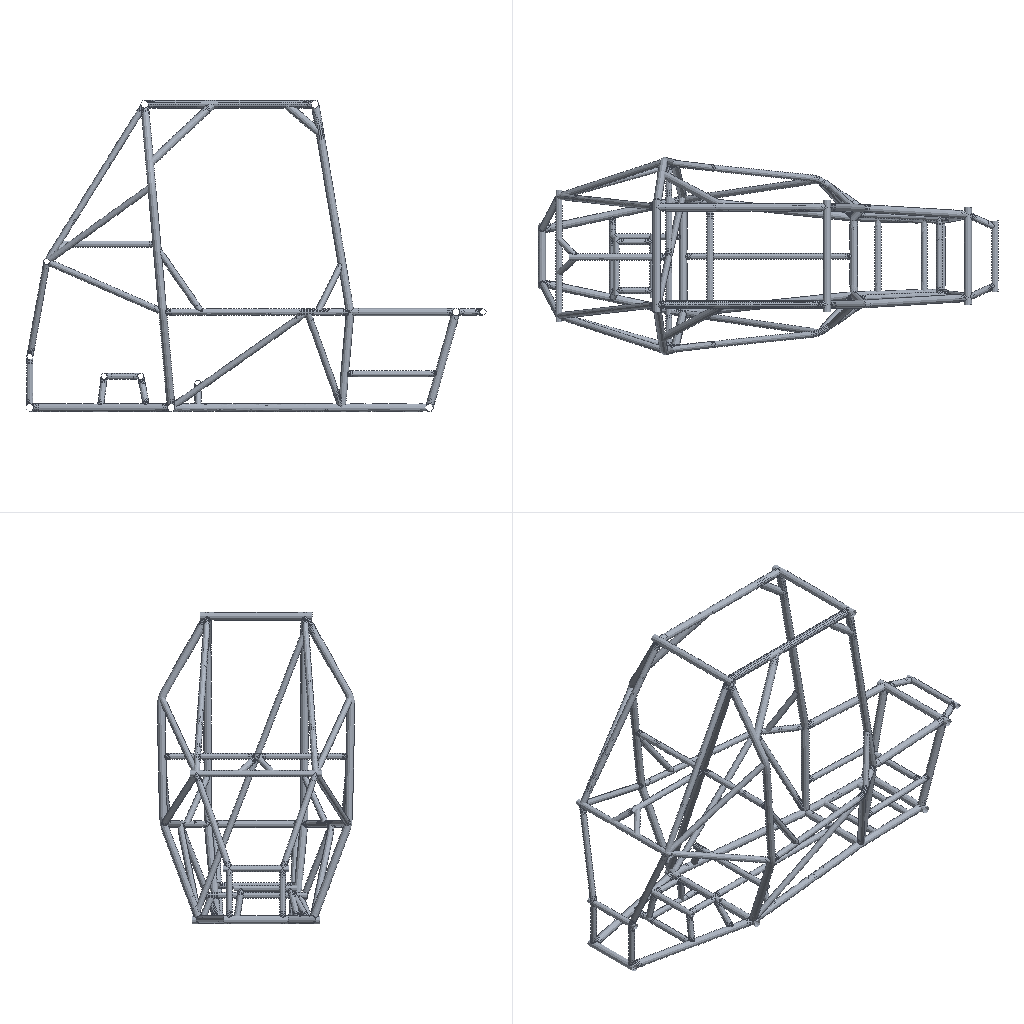Simulation study | ansys workbench
Set-up summary, first 98 of 221 lines:
category,name,step,type,value,unit,region
solver,ansys_workbench
units,mm-N-s-tonne (MPa),,stated,"/units,MPA"
analysis,LS1,,static
load_step,LS1,LS1,static,nsubst=1; time=1
mesh,nodes,,,59682
mesh,elements,,,95620
element_type,SHELL181,,,58416
element_type,CONTA174,,,18770
element_type,TARGE170,,,18398
element_type,CONTA177,,,36
material,4130?,,E,20500,tonne s^-2 mm^-1
material,4130?,,nu,0.29
material,4130?,,density,7.85e-09,tonne mm^-3
bc,"Elements for Body 1 ""fenxichejia0703-FreeParts|NONE""",model,fixed,[dofs=ALL n=3],,node list
bc,"Elements for Body 2 ""fenxichejia0703-FreeParts|NONE[2]""",model,fixed,[dofs=ALL n=3],,node list
bc,"Elements for Body 3 ""fenxichejia0703-FreeParts|NONE[3]""",model,fixed,[dofs=ALL n=3],,node list
bc,"Elements for Body 4 ""fenxichejia0703-FreeParts|NONE[4]""",model,fixed,[dofs=ALL n=3],,node list
bc,"Elements for Body 5 ""fenxichejia0703-FreeParts|NONE[5]""",model,fixed,[dofs=ALL n=3],,node list
bc,"Elements for Body 6 ""fenxichejia0703-FreeParts|NONE[6]""",model,fixed,[dofs=ALL n=3],,node list
bc,"Elements for Body 7 ""fenxichejia0703-FreeParts|NONE[7]""",model,fixed,[dofs=ALL n=3],,node list
bc,"Elements for Body 8 ""fenxichejia0703-FreeParts|NONE[8]""",model,fixed,[dofs=ALL n=3],,node list
bc,"Elements for Body 9 ""fenxichejia0703-FreeParts|NONE[9]""",model,fixed,[dofs=ALL n=3],,node list
bc,"Elements for Body 10 ""fenxichejia0703-FreeParts|NONE[10]""",model,fixed,[dofs=ALL n=3],,node list
bc,"Elements for Body 11 ""fenxichejia0703-FreeParts|NONE[11]""",model,fixed,[dofs=ALL n=3],,node list
bc,"Elements for Body 12 ""fenxichejia0703-FreeParts|NONE[12]""",model,fixed,[dofs=ALL n=3],,node list
bc,"Elements for Body 13 ""fenxichejia0703-FreeParts|NONE[13]""",model,fixed,[dofs=ALL n=3],,node list
bc,"Elements for Body 14 ""fenxichejia0703-FreeParts|NONE[14]""",model,fixed,[dofs=ALL n=3],,node list
bc,"Elements for Body 15 ""fenxichejia0703-FreeParts|NONE[15]""",model,fixed,[dofs=ALL n=3],,node list
bc,"Elements for Body 16 ""fenxichejia0703-FreeParts|NONE[16]""",model,fixed,[dofs=ALL n=3],,node list
bc,"Elements for Body 17 ""fenxichejia0703-FreeParts|NONE[17]""",model,fixed,[dofs=ALL n=3],,node list
bc,"Elements for Body 18 ""fenxichejia0703-FreeParts|NONE[18]""",model,fixed,[dofs=ALL n=3],,node list
bc,"Elements for Body 19 ""fenxichejia0703-FreeParts|NONE[19]""",model,fixed,[dofs=ALL n=3],,node list
bc,"Elements for Body 20 ""fenxichejia0703-FreeParts|NONE[20]""",model,fixed,[dofs=ALL n=3],,node list
bc,"Elements for Body 21 ""fenxichejia0703-FreeParts|NONE[21]""",model,fixed,[dofs=ALL n=3],,node list
bc,"Elements for Body 22 ""fenxichejia0703-FreeParts|NONE[22]""",model,fixed,[dofs=ALL n=3],,node list
bc,"Elements for Body 23 ""fenxichejia0703-FreeParts|NONE[23]""",model,fixed,[dofs=ALL n=3],,node list
bc,"Elements for Body 24 ""fenxichejia0703-FreeParts|NONE[24]""",model,fixed,[dofs=ALL n=3],,node list
bc,"Elements for Body 25 ""fenxichejia0703-FreeParts|NONE[25]""",model,fixed,[dofs=ALL n=3],,node list
bc,"Elements for Body 26 ""fenxichejia0703-FreeParts|NONE[26]""",model,fixed,[dofs=ALL n=3],,node list
bc,"Elements for Body 27 ""fenxichejia0703-FreeParts|NONE[27]""",model,fixed,[dofs=ALL n=3],,node list
bc,"Elements for Body 28 ""fenxichejia0703-FreeParts|NONE[28]""",model,fixed,[dofs=ALL n=3],,node list
bc,"Elements for Body 29 ""fenxichejia0703-FreeParts|NONE[29]""",model,fixed,[dofs=ALL n=3],,node list
bc,"Elements for Body 30 ""fenxichejia0703-FreeParts|NONE[30]""",model,fixed,[dofs=ALL n=3],,node list
bc,"Elements for Body 31 ""fenxichejia0703-FreeParts|NONE[31]""",model,fixed,[dofs=ALL n=3],,node list
bc,"Elements for Body 32 ""fenxichejia0703-FreeParts|NONE[32]""",model,fixed,[dofs=ALL n=3],,node list
bc,"Elements for Body 33 ""fenxichejia0703-FreeParts|NONE[33]""",model,fixed,[dofs=ALL n=3],,node list
bc,"Elements for Body 34 ""fenxichejia0703-FreeParts|NONE[34]""",model,fixed,[dofs=ALL n=3],,node list
bc,"Elements for Body 35 ""fenxichejia0703-FreeParts|NONE[35]""",model,fixed,[dofs=ALL n=3],,node list
bc,"Elements for Body 36 ""fenxichejia0703-FreeParts|NONE[36]""",model,fixed,[dofs=ALL n=3],,node list
bc,"Elements for Body 37 ""fenxichejia0703-FreeParts|NONE[37]""",model,fixed,[dofs=ALL n=3],,node list
bc,"Elements for Body 38 ""fenxichejia0703-FreeParts|NONE[38]""",model,fixed,[dofs=ALL n=3],,node list
bc,"Elements for Body 39 ""fenxichejia0703-FreeParts|NONE[39]""",model,fixed,[dofs=ALL n=3],,node list
bc,"Elements for Body 40 ""fenxichejia0703-FreeParts|NONE[40]""",model,fixed,[dofs=ALL n=3],,node list
bc,"Elements for Body 41 ""fenxichejia0703-FreeParts|NONE[41]""",model,fixed,[dofs=ALL n=3],,node list
bc,"Elements for Body 42 ""fenxichejia0703-FreeParts|NONE[42]""",model,fixed,[dofs=ALL n=3],,node list
bc,"Elements for Body 43 ""fenxichejia0703-FreeParts|NONE[43]""",model,fixed,[dofs=ALL n=3],,node list
bc,"Elements for Body 44 ""fenxichejia0703-FreeParts|NONE[44]""",model,fixed,[dofs=ALL n=3],,node list
bc,"Elements for Body 45 ""fenxichejia0703-FreeParts|NONE[45]""",model,fixed,[dofs=ALL n=3],,node list
bc,"Elements for Body 46 ""fenxichejia0703-FreeParts|NONE[46]""",model,fixed,[dofs=ALL n=3],,node list
bc,"Elements for Body 47 ""fenxichejia0703-FreeParts|NONE[47]""",model,fixed,[dofs=ALL n=3],,node list
bc,"Elements for Body 48 ""fenxichejia0703-FreeParts|NONE[48]""",model,fixed,[dofs=ALL n=3],,node list
bc,"Elements for Body 49 ""fenxichejia0703-FreeParts|NONE[49]""",model,fixed,[dofs=ALL n=3],,node list
bc,"Elements for Body 50 ""fenxichejia0703-FreeParts|NONE[50]""",model,fixed,[dofs=ALL n=3],,node list
bc,"Elements for Body 51 ""fenxichejia0703-FreeParts|NONE[51]""",model,fixed,[dofs=ALL n=3],,node list
bc,"Elements for Body 52 ""fenxichejia0703-FreeParts|NONE[52]""",model,fixed,[dofs=ALL n=3],,node list
bc,"Elements for Body 53 ""fenxichejia0703-FreeParts|NONE[53]""",model,fixed,[dofs=ALL n=3],,node list
bc,"Elements for Body 54 ""fenxichejia0703-FreeParts|NONE[54]""",model,fixed,[dofs=ALL n=3],,node list
bc,"Elements for Body 55 ""fenxichejia0703-FreeParts|NONE[55]""",model,fixed,[dofs=ALL n=3],,node list
bc,"Elements for Body 56 ""fenxichejia0703-FreeParts|NONE[56]""",model,fixed,[dofs=ALL n=3],,node list
bc,"Elements for Body 57 ""fenxichejia0703-FreeParts|NONE[57]""",model,fixed,[dofs=ALL n=3],,node list
bc,"Elements for Body 58 ""fenxichejia0703-FreeParts|NONE[58]""",model,fixed,[dofs=ALL n=3],,node list
bc,"Elements for Body 59 ""fenxichejia0703-FreeParts|NONE[59]""",model,fixed,[dofs=ALL n=3],,node list
bc,"Elements for Body 60 ""fenxichejia0703-FreeParts|NONE[60]""",model,fixed,[dofs=ALL n=3],,node list
bc,"Elements for Body 61 ""fenxichejia0703-FreeParts|NONE[61]""",model,fixed,[dofs=ALL n=3],,node list
bc,"Elements for Body 62 ""fenxichejia0703-FreeParts|NONE[62]""",model,fixed,[dofs=ALL n=3],,node list
bc,"Elements for Body 63 ""fenxichejia0703-FreeParts|NONE[63]""",model,fixed,[dofs=ALL n=3],,node list
bc,"Elements for Body 64 ""fenxichejia0703-FreeParts|NONE[64]""",model,fixed,[dofs=ALL n=3],,node list
bc,"Elements for Body 65 ""fenxichejia0703-FreeParts|NONE[65]""",model,fixed,[dofs=ALL n=3],,node list
bc,"Elements for Body 66 ""fenxichejia0703-FreeParts|NONE[66]""",model,fixed,[dofs=ALL n=3],,node list
bc,"Elements for Body 67 ""fenxichejia0703-FreeParts|NONE[67]""",model,fixed,[dofs=ALL n=3],,node list
bc,"Elements for Body 68 ""fenxichejia0703-FreeParts|NONE[68]""",model,fixed,[dofs=ALL n=3],,node list
bc,"Elements for Body 69 ""fenxichejia0703-FreeParts|NONE[69]""",model,fixed,[dofs=ALL n=3],,node list
bc,"Elements for Body 70 ""fenxichejia0703-FreeParts|NONE[70]""",model,fixed,[dofs=ALL n=3],,node list
bc,"Elements for Body 71 ""fenxichejia0703-FreeParts|NONE[71]""",model,fixed,[dofs=ALL n=3],,node list
bc,,LS1,prescribed uz,5 [dofs=UZ n=4],,node list
contact,Contact Region,,bonded (always),element=CONTA174
contact,Contact Region 2,,bonded (always),element=CONTA174
contact,Contact Region 3,,bonded (always),element=CONTA174
contact,Contact Region 4,,bonded (always),element=CONTA174
contact,Contact Region 5,,bonded (always),element=CONTA174
contact,Contact Region 6,,bonded (always),element=CONTA174
contact,Contact Region 7,,bonded (always),element=CONTA174
contact,Contact Region 8,,bonded (always),element=CONTA174
contact,Contact Region 9,,bonded (always),element=CONTA174
contact,Contact Region 10,,bonded (always),element=CONTA174
contact,Contact Region 11,,bonded (always),element=CONTA174
contact,Contact Region 12,,bonded (always),element=CONTA174
Ansys APDL input file, long lists of numbers shortened:
/batch
/config,noeldb,1     ! force off writing results to database
*get,_wallstrt,active,,time,wall
! ANSYS input file written by Workbench version 2021 R1
! File used for geometry attach:
/title,_______--____ (A5)
! ****** Begin Custom Load Command Snippet ******
/COM, ACT Extensions:
/COM,     LSDYNA, 2021.1
/COM,
! ****** End   Custom Load Command Snippet ******
*DIM,_wb_ProjectScratch_dir,string,248
_wb_ProjectScratch_dir(1) = ''
*DIM,_wb_SolverFiles_dir,string,248
_wb_SolverFiles_dir(1) = ''
*DIM,_wb_userfiles_dir,string,248
_wb_userfiles_dir(1) = ''
/com,--- Data in consistent NMM units. See Solving Units in the help system for more information.
/units,MPA
/nopr
/wb,file,start              !  signify a WB generated input file
/prep7
! Turn off shape checking because checks already performed inside WB mesher.
! See help system for more information.
SHPP,OFF,,NOWARN
/nolist
etcon,set             ! allow ANSYS to choose best KEYOP's for 180x elements, resets any applicable keyopt to MAPDL defaults
/com,*********** Nodes for the whole assembly ***********
nblock,3,,65645
(1i9,3e20.9e3)
        1     1.226998401E+02     1.799362606E+02     1.000000019E+02
! (59677 more lines like these left out)
-1
/com,*********** Nodes for all Remote Points ***********
nblock,3
(1i9,3e20.9e3)
    59679    -5.800208747E+02    -1.300000000E+02     6.838973832E-14
    59680    -5.800208747E+02     1.300000000E+02    -4.884981308E-14
    59681     1.060020881E+03    -1.800000000E+02    -2.451372438E-13
    59682     1.060020881E+03     1.800000000E+02     2.522426712E-13
-1
/wb,elem,start            !  set before creation of elements
/com,*********** Elements for Body 1 "fenxichejia0703-FreeParts|NONE" ***********
et,1,181
keyo,1,3,2
eblock,19,solid,,344
(19i9)
        1        1        1        1        0        0        0        0        4        0      199      457      341      467      467
! (343 more lines like these left out)
-1
/com,*********** Elements for Body 2 "fenxichejia0703-FreeParts|NONE[2]" ***********
et,2,181
keyo,2,3,2
eblock,19,solid,,220
(19i9)
        2        2        2        2        0        0        0        0        4        0     2766     2885     2887     3082     3082
! (219 more lines like these left out)
-1
/com,*********** Elements for Body 3 "fenxichejia0703-FreeParts|NONE[3]" ***********
et,3,181
keyo,3,3,2
eblock,19,solid,,992
(19i9)
        3        3        3        3        0        0        0        0        4        0    39705    41781    41416    41519    41419
! (991 more lines like these left out)
-1
/com,*********** Elements for Body 4 "fenxichejia0703-FreeParts|NONE[4]" ***********
et,4,181
keyo,4,3,2
eblock,19,solid,,978
(19i9)
        4        4        4        4        0        0        0        0        4        0    41902    43622    43598    43712    43712
! (977 more lines like these left out)
-1
/com,*********** Elements for Body 5 "fenxichejia0703-FreeParts|NONE[5]" ***********
et,5,181
keyo,5,3,2
eblock,19,solid,,572
(19i9)
        5        5        5        5        0        0        0        0        4        0    19833    20845    20860    20630    20630
! (571 more lines like these left out)
-1
! (66 more sections like these left out)
/wb,elem,end               !  done creating elements
/com,*********** Send User Defined Coordinate System(s) ***********
csys,0
toffst,273.15,  ! Temperature offset from absolute zero
/com,*********** Set Reference Temperature ***********
tref,22.
/wb,mat,start              !  starting to send materials
/com,*********** Send Materials ***********
MP,DENS,1,7.85e-09,	! tonne mm^-3
MP,EX,1,20500,	! tonne s^-2 mm^-1
MP,NUXY,1,0.29,
MP,DENS,2,7.85e-09,	! tonne mm^-3
! (209 more lines like these left out)
/wb,mat,end                !  done sending materials
/com,*********** Send Sheet Properties ***********
sectype,29,shell
secdata,3.
secoff,mid
sectype,30,shell
secdata,3.
secoff,mid
sectype,31,shell
secdata,3.
secoff,mid
sectype,32,shell
secdata,3.
secoff,mid
sectype,33,shell
secdata,3.
secoff,mid
sectype,34,shell
secdata,3.
secoff,mid
sectype,35,shell
secdata,3.
secoff,mid
sectype,36,shell
secdata,3.
secoff,mid
sectype,37,shell
secdata,3.
secoff,mid
sectype,38,shell
secdata,3.
secoff,mid
sectype,39,shell
secdata,3.
secoff,mid
sectype,40,shell
secdata,3.
secoff,mid
sectype,41,shell
secdata,3.
secoff,mid
sectype,42,shell
secdata,3.
secoff,mid
sectype,43,shell
secdata,3.
secoff,mid
sectype,44,shell
secdata,3.
secoff,mid
sectype,45,shell
secdata,3.
secoff,mid
sectype,46,shell
secdata,3.
secoff,mid
sectype,47,shell
secdata,3.
secoff,mid
sectype,48,shell
secdata,3.
secoff,mid
sectype,49,shell
secdata,3.
secoff,mid
sectype,50,shell
secdata,3.
secoff,mid
sectype,51,shell
secdata,3.
secoff,mid
sectype,1,shell
secdata,3.
secoff,mid
sectype,52,shell
secdata,3.
secoff,mid
sectype,53,shell
secdata,3.
secoff,mid
sectype,54,shell
! (147 more lines like these left out)
/wb,contact,start          !  starting to send contact
/com,*********** Create Contact "接触区域" ***********
/com,            Real Constant Set For Above Contact Is 73 & 72
*set,tid,73
*set,cid,72
r,tid
r,cid
et,tid,170
et,cid,174
eblock,10,,,78
(15i9)
    58421       73       73       73        0      277      283      285      285
! (77 more lines like these left out)
-1
eblock,10,,,78
(15i9)
    58499       72       72       72        0      277      283      285      285
! (77 more lines like these left out)
-1
eblock,10,,,40
(15i9)
    58577       72       73       72        0     3112     3043     3046     3046
! (39 more lines like these left out)
-1
eblock,10,,,40
(15i9)
    58617       73       72       73        0     3112     3043     3046     3046
! (39 more lines like these left out)
-1
keyo,cid,8,2               ! auto create asymmetric contact (from Program Controlled setting)
keyo,cid,10,0              ! adjust contact stiffness each NR iteration (from Program Controlled setting)
keyo,cid,12,5              ! bonded always
keyo,cid,18,1              ! small sliding turned on by application
keyo,cid,2,0               ! augmented Lagrange (from Program Controlled setting)
keyo,cid,4,0               ! on Gauss point (from Program Controlled setting)
keyo,cid,9,1               ! ignore initial gaps/penetration
keyo,cid,7,0               ! No Prediction
rmod,tid,3,10.      ! FKN
rmod,tid,5,0.       ! ICONT
rmod,tid,6,-6.067  ! PINB
rmod,tid,10,0.      ! CNOF
rmod,tid,12,0.      ! FKT
rmod,tid,36,234     ! WB DSID
rmod,cid,3,10.      ! FKN
rmod,cid,5,0.       ! ICONT
rmod,cid,6,-6.067  ! PINB
rmod,cid,10,0.      ! CNOF
rmod,cid,12,0.      ! FKT
rmod,cid,36,234     ! WB DSID
/com,*********** Create Contact "接触区域 2" ***********
/com,            Real Constant Set For Above Contact Is 75 & 74
*set,tid,75
*set,cid,74
r,tid
r,cid
et,tid,170
et,cid,174
eblock,10,,,41
(15i9)
    58657       75       75       75        0      464      383      326      327
! (40 more lines like these left out)
-1
eblock,10,,,41
(15i9)
    58698       74       74       74        0      464      383      326      327
! (40 more lines like these left out)
-1
eblock,10,,,32
(15i9)
    58739       74       75       74        0    23870    24089    23860    24099
! (31 more lines like these left out)
-1
eblock,10,,,32
(15i9)
    58771       75       74       75        0    23870    24089    23860    24099
! (31 more lines like these left out)
-1
keyo,cid,8,2               ! auto create asymmetric contact (from Program Controlled setting)
keyo,cid,10,0              ! adjust contact stiffness each NR iteration (from Program Controlled setting)
keyo,cid,12,5              ! bonded always
keyo,cid,18,1              ! small sliding turned on by application
keyo,cid,2,0               ! augmented Lagrange (from Program Controlled setting)
keyo,cid,4,0               ! on Gauss point (from Program Controlled setting)
keyo,cid,9,1               ! ignore initial gaps/penetration
keyo,cid,7,0               ! No Prediction
rmod,tid,3,10.      ! FKN
rmod,tid,5,0.       ! ICONT
rmod,tid,6,-6.067  ! PINB
rmod,tid,10,0.      ! CNOF
rmod,tid,12,0.      ! FKT
rmod,tid,36,237     ! WB DSID
rmod,cid,3,10.      ! FKN
rmod,cid,5,0.       ! ICONT
rmod,cid,6,-6.067  ! PINB
rmod,cid,10,0.      ! CNOF
rmod,cid,12,0.      ! FKT
rmod,cid,36,237     ! WB DSID
/com,*********** Create Contact "接触区域 3" ***********
/com,            Real Constant Set For Above Contact Is 77 & 76
*set,tid,77
*set,cid,76
r,tid
r,cid
et,tid,170
et,cid,174
eblock,10,,,76
(15i9)
    58803       77       77       77        0      226      225      228      228
! (75 more lines like these left out)
-1
eblock,10,,,76
(15i9)
    58879       76       76       76        0      226      225      228      228
! (75 more lines like these left out)
-1
eblock,10,,,111
(15i9)
    58955       76       77       76        0    35492    35870    35666    35665
! (110 more lines like these left out)
-1
eblock,10,,,111
(15i9)
    59066       77       76       77        0    35492    35870    35666    35665
! (110 more lines like these left out)
-1
keyo,cid,8,2               ! auto create asymmetric contact (from Program Controlled setting)
keyo,cid,10,0              ! adjust contact stiffness each NR iteration (from Program Controlled setting)
keyo,cid,12,5              ! bonded always
keyo,cid,18,1              ! small sliding turned on by application
keyo,cid,2,0               ! augmented Lagrange (from Program Controlled setting)
keyo,cid,4,0               ! on Gauss point (from Program Controlled setting)
keyo,cid,9,1               ! ignore initial gaps/penetration
keyo,cid,7,0               ! No Prediction
rmod,tid,3,10.      ! FKN
rmod,tid,5,0.       ! ICONT
rmod,tid,6,-6.067  ! PINB
rmod,tid,10,0.      ! CNOF
rmod,tid,12,0.      ! FKT
rmod,tid,36,240     ! WB DSID
rmod,cid,3,10.      ! FKN
rmod,cid,5,0.       ! ICONT
rmod,cid,6,-6.067  ! PINB
rmod,cid,10,0.      ! CNOF
rmod,cid,12,0.      ! FKT
rmod,cid,36,240     ! WB DSID
/com,*********** Create Contact "接触区域 4" ***********
/com,            Real Constant Set For Above Contact Is 79 & 78
*set,tid,79
*set,cid,78
r,tid
r,cid
et,tid,170
et,cid,174
eblock,10,,,70
(15i9)
    59177       79       79       79        0     3112     3043     3046     3046
! (69 more lines like these left out)
-1
eblock,10,,,70
(15i9)
    59247       78       78       78        0     3112     3043     3046     3046
! (69 more lines like these left out)
-1
eblock,10,,,88
(15i9)
    59317       78       79       78        0    24115    24398    24187    24186
! (87 more lines like these left out)
-1
eblock,10,,,88
(15i9)
    59405       79       78       79        0    24115    24398    24187    24186
! (87 more lines like these left out)
-1
keyo,cid,8,2               ! auto create asymmetric contact (from Program Controlled setting)
keyo,cid,10,0              ! adjust contact stiffness each NR iteration (from Program Controlled setting)
keyo,cid,12,5              ! bonded always
keyo,cid,18,1              ! small sliding turned on by application
keyo,cid,2,0               ! augmented Lagrange (from Program Controlled setting)
keyo,cid,4,0               ! on Gauss point (from Program Controlled setting)
keyo,cid,9,1               ! ignore initial gaps/penetration
keyo,cid,7,0               ! No Prediction
rmod,tid,3,10.      ! FKN
rmod,tid,5,0.       ! ICONT
rmod,tid,6,-6.067  ! PINB
rmod,tid,10,0.      ! CNOF
rmod,tid,12,0.      ! FKT
rmod,tid,36,243     ! WB DSID
rmod,cid,3,10.      ! FKN
rmod,cid,5,0.       ! ICONT
rmod,cid,6,-6.067  ! PINB
rmod,cid,10,0.      ! CNOF
rmod,cid,12,0.      ! FKT
rmod,cid,36,243     ! WB DSID
/com,*********** Create Contact "接触区域 5" ***********
/com,            Real Constant Set For Above Contact Is 81 & 80
*set,tid,81
*set,cid,80
r,tid
r,cid
et,tid,170
et,cid,174
eblock,10,,,68
(15i9)
    59493       81       81       81        0     2885     2887     3082     3082
! (67 more lines like these left out)
-1
eblock,10,,,68
(15i9)
    59561       80       80       80        0     2885     2887     3082     3082
! (67 more lines like these left out)
-1
eblock,10,,,106
(15i9)
    59629       80       81       80        0    35489    35493    35589    35588
! (105 more lines like these left out)
-1
eblock,10,,,106
(15i9)
    59735       81       80       81        0    35489    35493    35589    35588
! (105 more lines like these left out)
-1
keyo,cid,8,2               ! auto create asymmetric contact (from Program Controlled setting)
keyo,cid,10,0              ! adjust contact stiffness each NR iteration (from Program Controlled setting)
keyo,cid,12,5              ! bonded always
keyo,cid,18,1              ! small sliding turned on by application
keyo,cid,2,0               ! augmented Lagrange (from Program Controlled setting)
keyo,cid,4,0               ! on Gauss point (from Program Controlled setting)
keyo,cid,9,1               ! ignore initial gaps/penetration
keyo,cid,7,0               ! No Prediction
rmod,tid,3,10.      ! FKN
rmod,tid,5,0.       ! ICONT
rmod,tid,6,-6.067  ! PINB
rmod,tid,10,0.      ! CNOF
rmod,tid,12,0.      ! FKT
rmod,tid,36,246     ! WB DSID
rmod,cid,3,10.      ! FKN
rmod,cid,5,0.       ! ICONT
rmod,cid,6,-6.067  ! PINB
rmod,cid,10,0.      ! CNOF
rmod,cid,12,0.      ! FKT
rmod,cid,36,246     ! WB DSID
! (125 more sections like these left out)
/wb,contact,end            !  done creating contacts
/golist
/wb,load,start             !  starting to send loads
/com,*********** Create Remote Point "内部远程点" ***********
! -------- Remote Point Used by "远程位移" --------
*set,tid,333
*set,cid,332
et,cid,174
et,tid,170
keyo,tid,2,1               ! Don't fix the pilot node
keyo,tid,4,111111
keyo,cid,12,5              ! Bonded Contact
keyo,cid,4,1               ! Deformable RBE3 style load
keyo,cid,2,2               ! MPC style contact
eblock,10,,,372
(15i9)
    95217      332      332      332        0    15146    15183    15182    15145
! (371 more lines like these left out)
-1
*set,_npilot,59679
_npilot645=_npilot
type,tid
mat ,cid
real,cid
tshape,pilo
en,95589,_npilot
tshape
/com,*********** Create Remote Point "内部远程点 2" ***********
! -------- Remote Point Used by "远程位移 2" --------
*set,tid,335
*set,cid,334
et,cid,177
et,tid,170
keyo,tid,2,1               ! Don't fix the pilot node
keyo,tid,4,111111
keyo,cid,12,5              ! Bonded Contact
keyo,cid,4,1               ! Deformable RBE3 style load
keyo,cid,2,2               ! MPC style contact
eblock,10,,,12
(15i9)
    95590      334      334      334        0    15093    15135
! (11 more lines like these left out)
-1
*set,_npilot,59680
_npilot657=_npilot
type,tid
mat ,cid
real,cid
tshape,pilo
en,95602,_npilot
tshape
/com,*********** Create Remote Point "内部远程点 3" ***********
! -------- Remote Point Used by "远程位移 3" --------
*set,tid,337
*set,cid,336
et,cid,177
et,tid,170
keyo,tid,2,1               ! Don't fix the pilot node
keyo,tid,4,111111
keyo,cid,12,5              ! Bonded Contact
keyo,cid,4,1               ! Deformable RBE3 style load
keyo,cid,2,2               ! MPC style contact
eblock,10,,,12
(15i9)
    95603      336      336      336        0    16627    16680
! (11 more lines like these left out)
-1
*set,_npilot,59681
_npilot660=_npilot
type,tid
mat ,cid
real,cid
tshape,pilo
en,95615,_npilot
tshape
/com,*********** Create Remote Point "内部远程点 4" ***********
! -------- Remote Point Used by "远程位移 4" --------
*set,tid,339
*set,cid,338
et,cid,177
et,tid,170
keyo,tid,2,1               ! Don't fix the pilot node
keyo,tid,4,111111
keyo,cid,12,5              ! Bonded Contact
keyo,cid,4,1               ! Deformable RBE3 style load
keyo,cid,2,2               ! MPC style contact
eblock,10,,,12
(15i9)
    95616      338      338      338        0    16583    16685
! (11 more lines like these left out)
-1
*set,_npilot,59682
_npilot663=_npilot
type,tid
mat ,cid
real,cid
tshape,pilo
en,95628,_npilot
tshape
/com,*********** Construct Remote Displacement ***********
/com,*********** Construct Remote Displacement ***********
/com,*********** Construct Remote Displacement ***********
/com,*********** Construct Remote Displacement ***********
/COM,*** Create a component for all remote displacements ***
CMBLOCK,REMOTEDISPALL,NODE,        4
(8i10)
     59679     59680     59681     59682
et,340,14             ! spring element type
/com,*********** Construct Weak Springs, Prototype 1 ***********
*set,_delta,8.434
type,340
mat,341
real,341
r,341,9.98216507957579e-005
nsel,all
*get,_nspr,ndmx
_nspr=_nspr+1
esel,s,type,,1
nsle,s,active
*get,_minx,node,0,mnloc,x
*get,_miny,node,0,mnloc,y
*get,_minz,node,0,mnloc,z
*get,_maxx,node,0,mxloc,x
*get,_maxy,node,0,mxloc,y
*get,_maxz,node,0,mxloc,z
*dim,_ntets,arra,8
_ntets(1) = NODE(_minx,_miny,_minz)
_ntets(2) = NODE(_minx,_miny,_maxz)
_ntets(3) = NODE(_minx,_maxy,_minz)
_ntets(4) = NODE(_minx,_maxy,_maxz)
_ntets(5) = NODE(_maxx,_miny,_minz)
_ntets(6) = NODE(_maxx,_miny,_maxz)
_ntets(7) = NODE(_maxx,_maxy,_minz)
_ntets(8) = NODE(_maxx,_maxy,_maxz)
*do,_i,1,8
  n,_nspr,nx(_ntets(_i))+_delta,ny(_ntets(_i)),nz(_ntets(_i))
  e,_ntets(_i),_nspr
  d,_nspr,all
  _nspr=_nspr+1
  n,_nspr,nx(_ntets(_i)),ny(_ntets(_i))+_delta,nz(_ntets(_i))
  e,_ntets(_i),_nspr
  d,_nspr,all
  _nspr=_nspr+1
  n,_nspr,nx(_ntets(_i)),ny(_ntets(_i)),nz(_ntets(_i))+_delta
  e,_ntets(_i),_nspr
  d,_nspr,all
  _nspr=_nspr+1
*enddo
*set,_ntets
nsel,all
esel,all
/com,*********** Construct Weak Springs, Prototype 2 ***********
*set,_delta,8.259
type,340
mat,342
real,342
r,342,1.2338667019096e-004
nsel,all
*get,_nspr,ndmx
_nspr=_nspr+1
esel,s,type,,2
nsle,s,active
*get,_minx,node,0,mnloc,x
*get,_miny,node,0,mnloc,y
*get,_minz,node,0,mnloc,z
*get,_maxx,node,0,mxloc,x
*get,_maxy,node,0,mxloc,y
*get,_maxz,node,0,mxloc,z
*dim,_ntets,arra,8
_ntets(1) = NODE(_minx,_miny,_minz)
_ntets(2) = NODE(_minx,_miny,_maxz)
_ntets(3) = NODE(_minx,_maxy,_minz)
_ntets(4) = NODE(_minx,_maxy,_maxz)
_ntets(5) = NODE(_maxx,_miny,_minz)
_ntets(6) = NODE(_maxx,_miny,_maxz)
_ntets(7) = NODE(_maxx,_maxy,_minz)
_ntets(8) = NODE(_maxx,_maxy,_maxz)
*do,_i,1,8
  n,_nspr,nx(_ntets(_i))+_delta,ny(_ntets(_i)),nz(_ntets(_i))
  e,_ntets(_i),_nspr
  d,_nspr,all
  _nspr=_nspr+1
  n,_nspr,nx(_ntets(_i)),ny(_ntets(_i))+_delta,nz(_ntets(_i))
  e,_ntets(_i),_nspr
  d,_nspr,all
  _nspr=_nspr+1
  n,_nspr,nx(_ntets(_i)),ny(_ntets(_i)),nz(_ntets(_i))+_delta
  e,_ntets(_i),_nspr
  d,_nspr,all
  _nspr=_nspr+1
*enddo
*set,_ntets
nsel,all
esel,all
/com,*********** Construct Weak Springs, Prototype 3 ***********
*set,_delta,35.074
type,340
mat,343
real,343
r,343,1.68498675560958e-004
nsel,all
*get,_nspr,ndmx
_nspr=_nspr+1
esel,s,type,,3
nsle,s,active
*get,_minx,node,0,mnloc,x
*get,_miny,node,0,mnloc,y
*get,_minz,node,0,mnloc,z
*get,_maxx,node,0,mxloc,x
*get,_maxy,node,0,mxloc,y
*get,_maxz,node,0,mxloc,z
*dim,_ntets,arra,8
_ntets(1) = NODE(_minx,_miny,_minz)
_ntets(2) = NODE(_minx,_miny,_maxz)
_ntets(3) = NODE(_minx,_maxy,_minz)
_ntets(4) = NODE(_minx,_maxy,_maxz)
_ntets(5) = NODE(_maxx,_miny,_minz)
_ntets(6) = NODE(_maxx,_miny,_maxz)
_ntets(7) = NODE(_maxx,_maxy,_minz)
_ntets(8) = NODE(_maxx,_maxy,_maxz)
*do,_i,1,8
  n,_nspr,nx(_ntets(_i))+_delta,ny(_ntets(_i)),nz(_ntets(_i))
  e,_ntets(_i),_nspr
  d,_nspr,all
  _nspr=_nspr+1
  n,_nspr,nx(_ntets(_i)),ny(_ntets(_i))+_delta,nz(_ntets(_i))
  e,_ntets(_i),_nspr
  d,_nspr,all
  _nspr=_nspr+1
  n,_nspr,nx(_ntets(_i)),ny(_ntets(_i)),nz(_ntets(_i))+_delta
  e,_ntets(_i),_nspr
  d,_nspr,all
  _nspr=_nspr+1
*enddo
*set,_ntets
nsel,all
esel,all
/com,*********** Construct Weak Springs, Prototype 4 ***********
*set,_delta,35.074
type,340
mat,344
real,344
r,344,1.69411550265547e-004
nsel,all
*get,_nspr,ndmx
_nspr=_nspr+1
esel,s,type,,4
nsle,s,active
*get,_minx,node,0,mnloc,x
*get,_miny,node,0,mnloc,y
*get,_minz,node,0,mnloc,z
*get,_maxx,node,0,mxloc,x
*get,_maxy,node,0,mxloc,y
*get,_maxz,node,0,mxloc,z
*dim,_ntets,arra,8
_ntets(1) = NODE(_minx,_miny,_minz)
_ntets(2) = NODE(_minx,_miny,_maxz)
_ntets(3) = NODE(_minx,_maxy,_minz)
_ntets(4) = NODE(_minx,_maxy,_maxz)
_ntets(5) = NODE(_maxx,_miny,_minz)
_ntets(6) = NODE(_maxx,_miny,_maxz)
_ntets(7) = NODE(_maxx,_maxy,_minz)
_ntets(8) = NODE(_maxx,_maxy,_maxz)
*do,_i,1,8
  n,_nspr,nx(_ntets(_i))+_delta,ny(_ntets(_i)),nz(_ntets(_i))
  e,_ntets(_i),_nspr
  d,_nspr,all
  _nspr=_nspr+1
  n,_nspr,nx(_ntets(_i)),ny(_ntets(_i))+_delta,nz(_ntets(_i))
  e,_ntets(_i),_nspr
  d,_nspr,all
  _nspr=_nspr+1
  n,_nspr,nx(_ntets(_i)),ny(_ntets(_i)),nz(_ntets(_i))+_delta
  e,_ntets(_i),_nspr
  d,_nspr,all
  _nspr=_nspr+1
*enddo
*set,_ntets
nsel,all
esel,all
/com,*********** Construct Weak Springs, Prototype 5 ***********
*set,_delta,21.722
type,340
mat,345
real,345
r,345,1.6013463530714e-004
nsel,all
*get,_nspr,ndmx
_nspr=_nspr+1
esel,s,type,,5
nsle,s,active
*get,_minx,node,0,mnloc,x
*get,_miny,node,0,mnloc,y
*get,_minz,node,0,mnloc,z
*get,_maxx,node,0,mxloc,x
*get,_maxy,node,0,mxloc,y
*get,_maxz,node,0,mxloc,z
*dim,_ntets,arra,8
_ntets(1) = NODE(_minx,_miny,_minz)
_ntets(2) = NODE(_minx,_miny,_maxz)
_ntets(3) = NODE(_minx,_maxy,_minz)
_ntets(4) = NODE(_minx,_maxy,_maxz)
_ntets(5) = NODE(_maxx,_miny,_minz)
_ntets(6) = NODE(_maxx,_miny,_maxz)
_ntets(7) = NODE(_maxx,_maxy,_minz)
_ntets(8) = NODE(_maxx,_maxy,_maxz)
*do,_i,1,8
  n,_nspr,nx(_ntets(_i))+_delta,ny(_ntets(_i)),nz(_ntets(_i))
  e,_ntets(_i),_nspr
  d,_nspr,all
  _nspr=_nspr+1
  n,_nspr,nx(_ntets(_i)),ny(_ntets(_i))+_delta,nz(_ntets(_i))
  e,_ntets(_i),_nspr
  d,_nspr,all
  _nspr=_nspr+1
  n,_nspr,nx(_ntets(_i)),ny(_ntets(_i)),nz(_ntets(_i))+_delta
  e,_ntets(_i),_nspr
  d,_nspr,all
  _nspr=_nspr+1
*enddo
*set,_ntets
nsel,all
esel,all
! (66 more sections like these left out)
/wb,load,end               !  done creating loads
/com,--- Number of total nodes = %_numnode%
/com,--- Number of contact elements = 37204
/com,--- Number of spring elements = 1704
/com,--- Number of bearing elements = 0
/com,--- Number of solid elements = 58416
/com,--- Number of condensed parts = 0
/com,--- Number of total elements = %_numelem%
*get,_wallbsol,active,,time,wall
/com,****************************************************************************
/com,*************************    SOLUTION       ********************************
/com,****************************************************************************
/solu
antype,0                   ! static analysis
_thickRatio=  0     ! Ratio of thick parts in the model
eqsl,sparse,,,,,1
cntr,print,1               ! print out contact info and also make no initial contact an error
cntr,out,yes               ! write contact output to file.cmn due to many contact pairs present
dmpoption,emat,no             ! Don't combine emat file for DANSYS
dmpoption,esav,no             ! Don't combine esav file for DANSYS
nldiag,cont,iter           ! print out contact info each equilibrium iteration
rescontrol,,none                 ! Do not keep any restart files
/com,****************************************************
/com,******************* SOLVE FOR LS 1 OF 1 ****************
d,59679,uz,5.
d,59680,uz,-5.
d,59681,uz,-5.
d,59682,uz,5.
/nopr
/gopr
/nolist
nsub,1,1,1
time,1.
outres,erase
outres,all,none
outres,nsol,all,
outres,rsol,all
outres,eangl,all
outres,etmp,all
outres,veng,all
outres,strs,all,
outres,epel,all,
outres,eppl,all,
outres,cont,all,
! *********** WB SOLVE COMMAND ***********
! check interactive state
*get,ANSINTER_,active,,int
*if,ANSINTER_,ne,0,then
/eof
*endif
solve
/com *************** Write FE CONNECTORS *********
CEWRITE,file,ce,,INTE
/com,****************************************************
/com,*************** FINISHED SOLVE FOR LS 1 *************
*get,_wallasol,active,,time,wall
/nopr
*get,_numnode,node,0,count
*get,_numelem,elem,0,count
*get, _MAXELEMNUM, elem, 0, NUM, MAX
*get, _MAXNODENUM, node, 0, NUM, MAX,,,INTERNAL
*get, _MAXELEMTYPE, etyp, 0, NUM, MAX
*get, _MAXREALCONST, real, 0, NUM, MAX
/gopr
/post1
xmlo,ENCODING,ISO-8859-1
xmlo,parm
/xml,parm,xml
fini
/gopr
*get,_walldone,active,,time,wall
_preptime=(_wallbsol-_wallstrt)*3600
_solvtime=(_wallasol-_wallbsol)*3600
_posttime=(_walldone-_wallasol)*3600
_totaltim=(_walldone-_wallstrt)*3600
*get,_dlbratio,active,0,solu,dlbr
*get,_combtime,active,0,solu,comb
/com,--- Total number of nodes = %_numnode%
/com,--- Total number of elements = %_numelem%
/com,--- Element load balance ratio = %_dlbratio%
/com,--- Time to combine distributed files = %_combtime%
/wb,file,end               ! done with WB generated input
Results summary:
result,analyses[0].index,,,1
result,analyses[0].system,,,SYS
result,analyses[0].deck,,,deck.dat
result,analyses[0].solve_status,,,completed
result,analyses[0].analysis_type,,,static
result,analyses[0].physics,,,mechanical
result,analyses[0].unit_system,,,"NMM: mm, ton, N, s, mV, mA, degC"
result,analyses[0].n_sets,,,1
result,analyses[0].load_steps[0].set,set=1,,1
result,analyses[0].load_steps[0].time_or_freq,set=1,,1
result,analyses[0].load_steps[0].max_displacement_magnitude,set=1,,5.729
result,analyses[0].load_steps[0].max_von_mises_nodal,set=1,,266.819
result,analyses[0].load_steps[0].reaction_force_sum_xyz[1],set=1,,4.09634e-05
result,analyses[0].load_steps[0].reaction_force_sum_xyz[2],set=1,,0.0001689
result,analyses[0].load_steps[0].reaction_force_sum_xyz[3],set=1,,-8.13396e-06
result,geometry_export[0][0],,,.step
result,geometry_export[0][1],,,ok
result,geometry_export[0][2],,,76